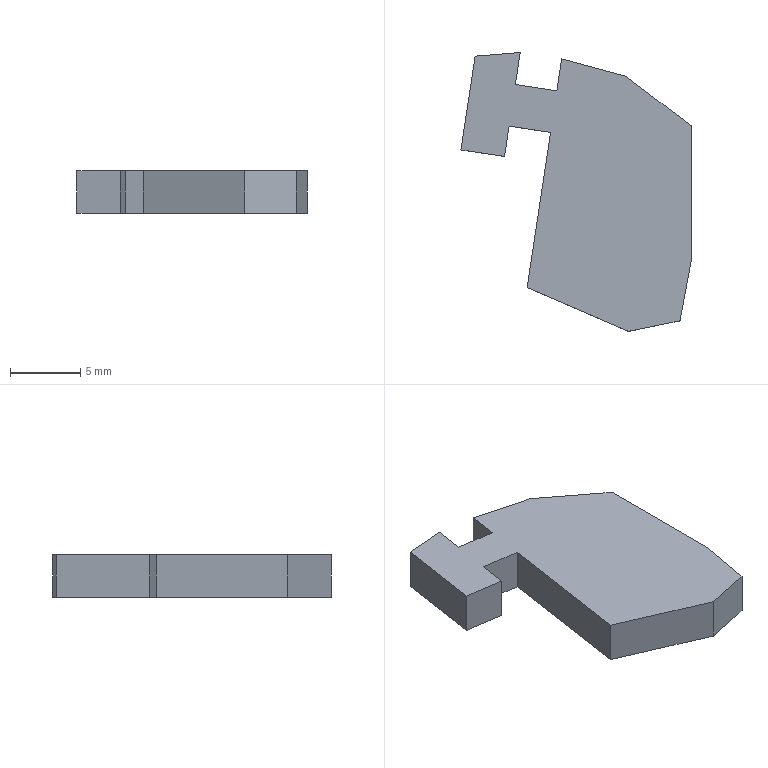Part | SolidWorks | features BaseBody 1 | 1 solid | 17 faces | box 16.417 x 19.898 x 3 mm | volume 620.666 mm3 | plane 17
STEP:
#1=CARTESIAN_POINT('',(6.476,-7.983,-1.5));
#2=VERTEX_POINT('',#1);
#3=CARTESIAN_POINT('',(7.263,-3.747,-1.5));
#4=VERTEX_POINT('',#3);
#5=CARTESIAN_POINT('',(6.476,-7.983,-1.5));
#6=DIRECTION('',(0.1826,0.9832,0.));
#7=VECTOR('',#6,1000.);
#8=LINE('',#5,#7);
#9=EDGE_CURVE('',#2,#4,#8,.T.);
#10=ORIENTED_EDGE('',*,*,#9,.F.);
#11=CARTESIAN_POINT('',(2.819,-8.745,-1.5));
#12=VERTEX_POINT('',#11);
#13=CARTESIAN_POINT('',(2.819,-8.745,-1.5));
#14=DIRECTION('',(0.9789,0.2042,0.));
#15=VECTOR('',#14,1000.);
#16=LINE('',#13,#15);
#17=EDGE_CURVE('',#12,#2,#16,.T.);
#18=ORIENTED_EDGE('',*,*,#17,.F.);
#19=CARTESIAN_POINT('',(-4.433,-5.618,-1.5));
#20=VERTEX_POINT('',#19);
#21=CARTESIAN_POINT('',(-4.433,-5.618,-1.5));
#22=DIRECTION('',(0.9183,-0.3959,0.));
#23=VECTOR('',#22,1000.);
#24=LINE('',#21,#23);
#25=EDGE_CURVE('',#20,#12,#24,.T.);
#26=ORIENTED_EDGE('',*,*,#25,.F.);
#27=CARTESIAN_POINT('',(-2.759,5.455,-1.5));
#28=VERTEX_POINT('',#27);
#29=CARTESIAN_POINT('',(-2.759,5.455,-1.5));
#30=DIRECTION('',(-0.1495,-0.9888,0.));
#31=VECTOR('',#30,1000.);
#32=LINE('',#29,#31);
#33=EDGE_CURVE('',#28,#20,#32,.T.);
#34=ORIENTED_EDGE('',*,*,#33,.F.);
#35=CARTESIAN_POINT('',(-5.721,5.903,-1.5));
#36=VERTEX_POINT('',#35);
#37=CARTESIAN_POINT('',(-5.721,5.903,-1.5));
#38=DIRECTION('',(0.9888,-0.1495,0.));
#39=VECTOR('',#38,1000.);
#40=LINE('',#37,#39);
#41=EDGE_CURVE('',#36,#28,#40,.T.);
#42=ORIENTED_EDGE('',*,*,#41,.F.);
#43=CARTESIAN_POINT('',(-6.049,3.738,-1.5));
#44=VERTEX_POINT('',#43);
#45=CARTESIAN_POINT('',(-6.049,3.738,-1.5));
#46=DIRECTION('',(0.1495,0.9888,0.));
#47=VECTOR('',#46,1000.);
#48=LINE('',#45,#47);
#49=EDGE_CURVE('',#44,#36,#48,.T.);
#50=ORIENTED_EDGE('',*,*,#49,.F.);
#51=CARTESIAN_POINT('',(-9.154,4.206,-1.5));
#52=VERTEX_POINT('',#51);
#53=CARTESIAN_POINT('',(-9.154,4.206,-1.5));
#54=DIRECTION('',(0.9889,-0.1488,0.));
#55=VECTOR('',#54,1000.);
#56=LINE('',#53,#55);
#57=EDGE_CURVE('',#52,#44,#56,.T.);
#58=ORIENTED_EDGE('',*,*,#57,.F.);
#59=CARTESIAN_POINT('',(-8.143,10.895,-1.5));
#60=VERTEX_POINT('',#59);
#61=CARTESIAN_POINT('',(-8.143,10.895,-1.5));
#62=DIRECTION('',(-0.1495,-0.9888,0.));
#63=VECTOR('',#62,1000.);
#64=LINE('',#61,#63);
#65=EDGE_CURVE('',#60,#52,#64,.T.);
#66=ORIENTED_EDGE('',*,*,#65,.F.);
#67=CARTESIAN_POINT('',(-4.928,11.153,-1.5));
#68=VERTEX_POINT('',#67);
#69=CARTESIAN_POINT('',(-4.928,11.153,-1.5));
#70=DIRECTION('',(-0.9968,-0.08003,0.));
#71=VECTOR('',#70,1000.);
#72=LINE('',#69,#71);
#73=EDGE_CURVE('',#68,#60,#72,.T.);
#74=ORIENTED_EDGE('',*,*,#73,.F.);
#75=CARTESIAN_POINT('',(-5.273,8.869,-1.5));
#76=VERTEX_POINT('',#75);
#77=CARTESIAN_POINT('',(-5.273,8.869,-1.5));
#78=DIRECTION('',(0.1495,0.9888,0.));
#79=VECTOR('',#78,1000.);
#80=LINE('',#77,#79);
#81=EDGE_CURVE('',#76,#68,#80,.T.);
#82=ORIENTED_EDGE('',*,*,#81,.F.);
#83=CARTESIAN_POINT('',(-2.31,8.421,-1.5));
#84=VERTEX_POINT('',#83);
#85=CARTESIAN_POINT('',(-2.31,8.421,-1.5));
#86=DIRECTION('',(-0.9888,0.1495,0.));
#87=VECTOR('',#86,1000.);
#88=LINE('',#85,#87);
#89=EDGE_CURVE('',#84,#76,#88,.T.);
#90=ORIENTED_EDGE('',*,*,#89,.F.);
#91=CARTESIAN_POINT('',(-1.965,10.705,-1.5));
#92=VERTEX_POINT('',#91);
#93=CARTESIAN_POINT('',(-2.31,8.421,-1.5));
#94=DIRECTION('',(0.1495,0.9888,0.));
#95=VECTOR('',#94,1000.);
#96=LINE('',#93,#95);
#97=EDGE_CURVE('',#84,#92,#96,.T.);
#98=ORIENTED_EDGE('',*,*,#97,.T.);
#99=CARTESIAN_POINT('',(2.616,9.465,-1.5));
#100=VERTEX_POINT('',#99);
#101=CARTESIAN_POINT('',(2.616,9.465,-1.5));
#102=DIRECTION('',(-0.9652,0.2614,0.));
#103=VECTOR('',#102,1000.);
#104=LINE('',#101,#103);
#105=EDGE_CURVE('',#100,#92,#104,.T.);
#106=ORIENTED_EDGE('',*,*,#105,.F.);
#107=CARTESIAN_POINT('',(7.263,5.919,-1.5));
#108=VERTEX_POINT('',#107);
#109=CARTESIAN_POINT('',(7.263,5.919,-1.5));
#110=DIRECTION('',(-0.795,0.6067,0.));
#111=VECTOR('',#110,1000.);
#112=LINE('',#109,#111);
#113=EDGE_CURVE('',#108,#100,#112,.T.);
#114=ORIENTED_EDGE('',*,*,#113,.F.);
#115=CARTESIAN_POINT('',(7.263,-3.747,-1.5));
#116=DIRECTION('',(0.,1.,0.));
#117=VECTOR('',#116,1000.);
#118=LINE('',#115,#117);
#119=EDGE_CURVE('',#4,#108,#118,.T.);
#120=ORIENTED_EDGE('',*,*,#119,.F.);
#121=EDGE_LOOP('',(#10,#18,#26,#34,#42,#50,#58,#66,#74,#82,#90,#98,#106,#114,#120));
#122=FACE_OUTER_BOUND('',#121,.T.);
#123=CARTESIAN_POINT('',(0.,0.,-1.5));
#124=DIRECTION('',(0.,0.,1.));
#125=DIRECTION('',(1.,0.,0.));
#126=AXIS2_PLACEMENT_3D('',#123,#124,#125);
#127=PLANE('',#126);
#128=ADVANCED_FACE('',(#122),#127,.F.);
#129=CARTESIAN_POINT('',(6.476,-7.983,1.5));
#130=VERTEX_POINT('',#129);
#131=CARTESIAN_POINT('',(7.263,-3.747,1.5));
#132=VERTEX_POINT('',#131);
#133=CARTESIAN_POINT('',(6.476,-7.983,1.5));
#134=DIRECTION('',(0.1826,0.9832,0.));
#135=VECTOR('',#134,1000.);
#136=LINE('',#133,#135);
#137=EDGE_CURVE('',#130,#132,#136,.T.);
#138=ORIENTED_EDGE('',*,*,#137,.T.);
#139=CARTESIAN_POINT('',(7.263,5.919,1.5));
#140=VERTEX_POINT('',#139);
#141=CARTESIAN_POINT('',(7.263,-3.747,1.5));
#142=DIRECTION('',(0.,1.,0.));
#143=VECTOR('',#142,1000.);
#144=LINE('',#141,#143);
#145=EDGE_CURVE('',#132,#140,#144,.T.);
#146=ORIENTED_EDGE('',*,*,#145,.T.);
#147=CARTESIAN_POINT('',(2.616,9.465,1.5));
#148=VERTEX_POINT('',#147);
#149=CARTESIAN_POINT('',(7.263,5.919,1.5));
#150=DIRECTION('',(-0.795,0.6067,0.));
#151=VECTOR('',#150,1000.);
#152=LINE('',#149,#151);
#153=EDGE_CURVE('',#140,#148,#152,.T.);
#154=ORIENTED_EDGE('',*,*,#153,.T.);
#155=CARTESIAN_POINT('',(-1.965,10.705,1.5));
#156=VERTEX_POINT('',#155);
#157=CARTESIAN_POINT('',(2.616,9.465,1.5));
#158=DIRECTION('',(-0.9652,0.2614,0.));
#159=VECTOR('',#158,1000.);
#160=LINE('',#157,#159);
#161=EDGE_CURVE('',#148,#156,#160,.T.);
#162=ORIENTED_EDGE('',*,*,#161,.T.);
#163=CARTESIAN_POINT('',(-2.31,8.421,1.5));
#164=VERTEX_POINT('',#163);
#165=CARTESIAN_POINT('',(-2.31,8.421,1.5));
#166=DIRECTION('',(0.1495,0.9888,0.));
#167=VECTOR('',#166,1000.);
#168=LINE('',#165,#167);
#169=EDGE_CURVE('',#164,#156,#168,.T.);
#170=ORIENTED_EDGE('',*,*,#169,.F.);
#171=CARTESIAN_POINT('',(-5.273,8.869,1.5));
#172=VERTEX_POINT('',#171);
#173=CARTESIAN_POINT('',(-2.31,8.421,1.5));
#174=DIRECTION('',(-0.9888,0.1495,0.));
#175=VECTOR('',#174,1000.);
#176=LINE('',#173,#175);
#177=EDGE_CURVE('',#164,#172,#176,.T.);
#178=ORIENTED_EDGE('',*,*,#177,.T.);
#179=CARTESIAN_POINT('',(-4.928,11.153,1.5));
#180=VERTEX_POINT('',#179);
#181=CARTESIAN_POINT('',(-5.273,8.869,1.5));
#182=DIRECTION('',(0.1495,0.9888,0.));
#183=VECTOR('',#182,1000.);
#184=LINE('',#181,#183);
#185=EDGE_CURVE('',#172,#180,#184,.T.);
#186=ORIENTED_EDGE('',*,*,#185,.T.);
#187=CARTESIAN_POINT('',(-8.143,10.895,1.5));
#188=VERTEX_POINT('',#187);
#189=CARTESIAN_POINT('',(-4.928,11.153,1.5));
#190=DIRECTION('',(-0.9968,-0.08003,0.));
#191=VECTOR('',#190,1000.);
#192=LINE('',#189,#191);
#193=EDGE_CURVE('',#180,#188,#192,.T.);
#194=ORIENTED_EDGE('',*,*,#193,.T.);
#195=CARTESIAN_POINT('',(-9.154,4.206,1.5));
#196=VERTEX_POINT('',#195);
#197=CARTESIAN_POINT('',(-8.143,10.895,1.5));
#198=DIRECTION('',(-0.1495,-0.9888,0.));
#199=VECTOR('',#198,1000.);
#200=LINE('',#197,#199);
#201=EDGE_CURVE('',#188,#196,#200,.T.);
#202=ORIENTED_EDGE('',*,*,#201,.T.);
#203=CARTESIAN_POINT('',(-6.049,3.738,1.5));
#204=VERTEX_POINT('',#203);
#205=CARTESIAN_POINT('',(-9.154,4.206,1.5));
#206=DIRECTION('',(0.9889,-0.1488,0.));
#207=VECTOR('',#206,1000.);
#208=LINE('',#205,#207);
#209=EDGE_CURVE('',#196,#204,#208,.T.);
#210=ORIENTED_EDGE('',*,*,#209,.T.);
#211=CARTESIAN_POINT('',(-5.721,5.903,1.5));
#212=VERTEX_POINT('',#211);
#213=CARTESIAN_POINT('',(-6.049,3.738,1.5));
#214=DIRECTION('',(0.1495,0.9888,0.));
#215=VECTOR('',#214,1000.);
#216=LINE('',#213,#215);
#217=EDGE_CURVE('',#204,#212,#216,.T.);
#218=ORIENTED_EDGE('',*,*,#217,.T.);
#219=CARTESIAN_POINT('',(-2.759,5.455,1.5));
#220=VERTEX_POINT('',#219);
#221=CARTESIAN_POINT('',(-5.721,5.903,1.5));
#222=DIRECTION('',(0.9888,-0.1495,0.));
#223=VECTOR('',#222,1000.);
#224=LINE('',#221,#223);
#225=EDGE_CURVE('',#212,#220,#224,.T.);
#226=ORIENTED_EDGE('',*,*,#225,.T.);
#227=CARTESIAN_POINT('',(-4.433,-5.618,1.5));
#228=VERTEX_POINT('',#227);
#229=CARTESIAN_POINT('',(-2.759,5.455,1.5));
#230=DIRECTION('',(-0.1495,-0.9888,0.));
#231=VECTOR('',#230,1000.);
#232=LINE('',#229,#231);
#233=EDGE_CURVE('',#220,#228,#232,.T.);
#234=ORIENTED_EDGE('',*,*,#233,.T.);
#235=CARTESIAN_POINT('',(2.819,-8.745,1.5));
#236=VERTEX_POINT('',#235);
#237=CARTESIAN_POINT('',(-4.433,-5.618,1.5));
#238=DIRECTION('',(0.9183,-0.3959,0.));
#239=VECTOR('',#238,1000.);
#240=LINE('',#237,#239);
#241=EDGE_CURVE('',#228,#236,#240,.T.);
#242=ORIENTED_EDGE('',*,*,#241,.T.);
#243=CARTESIAN_POINT('',(2.819,-8.745,1.5));
#244=DIRECTION('',(0.9789,0.2042,0.));
#245=VECTOR('',#244,1000.);
#246=LINE('',#243,#245);
#247=EDGE_CURVE('',#236,#130,#246,.T.);
#248=ORIENTED_EDGE('',*,*,#247,.T.);
#249=EDGE_LOOP('',(#138,#146,#154,#162,#170,#178,#186,#194,#202,#210,#218,#226,#234,#242,#248));
#250=FACE_OUTER_BOUND('',#249,.T.);
#251=CARTESIAN_POINT('',(0.,0.,1.5));
#252=DIRECTION('',(0.,0.,1.));
#253=DIRECTION('',(1.,0.,0.));
#254=AXIS2_PLACEMENT_3D('',#251,#252,#253);
#255=PLANE('',#254);
#256=ADVANCED_FACE('',(#250),#255,.T.);
#257=ORIENTED_EDGE('',*,*,#17,.T.);
#258=CARTESIAN_POINT('',(6.476,-7.983,1.5));
#259=DIRECTION('',(0.,0.,-1.));
#260=VECTOR('',#259,1000.);
#261=LINE('',#258,#260);
#262=EDGE_CURVE('',#130,#2,#261,.T.);
#263=ORIENTED_EDGE('',*,*,#262,.F.);
#264=ORIENTED_EDGE('',*,*,#247,.F.);
#265=CARTESIAN_POINT('',(2.819,-8.745,1.5));
#266=DIRECTION('',(0.,0.,-1.));
#267=VECTOR('',#266,1000.);
#268=LINE('',#265,#267);
#269=EDGE_CURVE('',#236,#12,#268,.T.);
#270=ORIENTED_EDGE('',*,*,#269,.T.);
#271=EDGE_LOOP('',(#257,#263,#264,#270));
#272=FACE_OUTER_BOUND('',#271,.T.);
#273=CARTESIAN_POINT('',(2.819,-8.745,1.5));
#274=DIRECTION('',(-0.2042,0.9789,0.));
#275=DIRECTION('',(0.,0.,1.));
#276=AXIS2_PLACEMENT_3D('',#273,#274,#275);
#277=PLANE('',#276);
#278=ADVANCED_FACE('',(#272),#277,.F.);
#279=ORIENTED_EDGE('',*,*,#25,.T.);
#280=ORIENTED_EDGE('',*,*,#269,.F.);
#281=ORIENTED_EDGE('',*,*,#241,.F.);
#282=CARTESIAN_POINT('',(-4.433,-5.618,1.5));
#283=DIRECTION('',(0.,0.,-1.));
#284=VECTOR('',#283,1000.);
#285=LINE('',#282,#284);
#286=EDGE_CURVE('',#228,#20,#285,.T.);
#287=ORIENTED_EDGE('',*,*,#286,.T.);
#288=EDGE_LOOP('',(#279,#280,#281,#287));
#289=FACE_OUTER_BOUND('',#288,.T.);
#290=CARTESIAN_POINT('',(-4.433,-5.618,1.5));
#291=DIRECTION('',(0.3959,0.9183,0.));
#292=DIRECTION('',(0.,0.,-1.));
#293=AXIS2_PLACEMENT_3D('',#290,#291,#292);
#294=PLANE('',#293);
#295=ADVANCED_FACE('',(#289),#294,.F.);
#296=ORIENTED_EDGE('',*,*,#33,.T.);
#297=ORIENTED_EDGE('',*,*,#286,.F.);
#298=ORIENTED_EDGE('',*,*,#233,.F.);
#299=CARTESIAN_POINT('',(-2.759,5.455,1.5));
#300=DIRECTION('',(0.,0.,-1.));
#301=VECTOR('',#300,1000.);
#302=LINE('',#299,#301);
#303=EDGE_CURVE('',#220,#28,#302,.T.);
#304=ORIENTED_EDGE('',*,*,#303,.T.);
#305=EDGE_LOOP('',(#296,#297,#298,#304));
#306=FACE_OUTER_BOUND('',#305,.T.);
#307=CARTESIAN_POINT('',(-2.759,5.455,1.5));
#308=DIRECTION('',(0.9888,-0.1495,0.));
#309=DIRECTION('',(0.,0.,-1.));
#310=AXIS2_PLACEMENT_3D('',#307,#308,#309);
#311=PLANE('',#310);
#312=ADVANCED_FACE('',(#306),#311,.F.);
#313=ORIENTED_EDGE('',*,*,#41,.T.);
#314=ORIENTED_EDGE('',*,*,#303,.F.);
#315=ORIENTED_EDGE('',*,*,#225,.F.);
#316=CARTESIAN_POINT('',(-5.721,5.903,1.5));
#317=DIRECTION('',(0.,0.,-1.));
#318=VECTOR('',#317,1000.);
#319=LINE('',#316,#318);
#320=EDGE_CURVE('',#212,#36,#319,.T.);
#321=ORIENTED_EDGE('',*,*,#320,.T.);
#322=EDGE_LOOP('',(#313,#314,#315,#321));
#323=FACE_OUTER_BOUND('',#322,.T.);
#324=CARTESIAN_POINT('',(-5.721,5.903,1.5));
#325=DIRECTION('',(0.1495,0.9888,0.));
#326=DIRECTION('',(0.,0.,-1.));
#327=AXIS2_PLACEMENT_3D('',#324,#325,#326);
#328=PLANE('',#327);
#329=ADVANCED_FACE('',(#323),#328,.F.);
#330=ORIENTED_EDGE('',*,*,#49,.T.);
#331=ORIENTED_EDGE('',*,*,#320,.F.);
#332=ORIENTED_EDGE('',*,*,#217,.F.);
#333=CARTESIAN_POINT('',(-6.049,3.738,1.5));
#334=DIRECTION('',(0.,0.,-1.));
#335=VECTOR('',#334,1000.);
#336=LINE('',#333,#335);
#337=EDGE_CURVE('',#204,#44,#336,.T.);
#338=ORIENTED_EDGE('',*,*,#337,.T.);
#339=EDGE_LOOP('',(#330,#331,#332,#338));
#340=FACE_OUTER_BOUND('',#339,.T.);
#341=CARTESIAN_POINT('',(-6.049,3.738,1.5));
#342=DIRECTION('',(-0.9888,0.1495,0.));
#343=DIRECTION('',(0.,0.,1.));
#344=AXIS2_PLACEMENT_3D('',#341,#342,#343);
#345=PLANE('',#344);
#346=ADVANCED_FACE('',(#340),#345,.F.);
#347=ORIENTED_EDGE('',*,*,#57,.T.);
#348=ORIENTED_EDGE('',*,*,#337,.F.);
#349=ORIENTED_EDGE('',*,*,#209,.F.);
#350=CARTESIAN_POINT('',(-9.154,4.206,1.5));
#351=DIRECTION('',(0.,0.,-1.));
#352=VECTOR('',#351,1000.);
#353=LINE('',#350,#352);
#354=EDGE_CURVE('',#196,#52,#353,.T.);
#355=ORIENTED_EDGE('',*,*,#354,.T.);
#356=EDGE_LOOP('',(#347,#348,#349,#355));
#357=FACE_OUTER_BOUND('',#356,.T.);
#358=CARTESIAN_POINT('',(-9.154,4.206,1.5));
#359=DIRECTION('',(0.1488,0.9889,0.));
#360=DIRECTION('',(0.,0.,-1.));
#361=AXIS2_PLACEMENT_3D('',#358,#359,#360);
#362=PLANE('',#361);
#363=ADVANCED_FACE('',(#357),#362,.F.);
#364=ORIENTED_EDGE('',*,*,#65,.T.);
#365=ORIENTED_EDGE('',*,*,#354,.F.);
#366=ORIENTED_EDGE('',*,*,#201,.F.);
#367=CARTESIAN_POINT('',(-8.143,10.895,1.5));
#368=DIRECTION('',(0.,0.,-1.));
#369=VECTOR('',#368,1000.);
#370=LINE('',#367,#369);
#371=EDGE_CURVE('',#188,#60,#370,.T.);
#372=ORIENTED_EDGE('',*,*,#371,.T.);
#373=EDGE_LOOP('',(#364,#365,#366,#372));
#374=FACE_OUTER_BOUND('',#373,.T.);
#375=CARTESIAN_POINT('',(-8.143,10.895,1.5));
#376=DIRECTION('',(0.9888,-0.1495,0.));
#377=DIRECTION('',(0.,0.,-1.));
#378=AXIS2_PLACEMENT_3D('',#375,#376,#377);
#379=PLANE('',#378);
#380=ADVANCED_FACE('',(#374),#379,.F.);
#381=ORIENTED_EDGE('',*,*,#73,.T.);
#382=ORIENTED_EDGE('',*,*,#371,.F.);
#383=ORIENTED_EDGE('',*,*,#193,.F.);
#384=CARTESIAN_POINT('',(-4.928,11.153,1.5));
#385=DIRECTION('',(0.,0.,-1.));
#386=VECTOR('',#385,1000.);
#387=LINE('',#384,#386);
#388=EDGE_CURVE('',#180,#68,#387,.T.);
#389=ORIENTED_EDGE('',*,*,#388,.T.);
#390=EDGE_LOOP('',(#381,#382,#383,#389));
#391=FACE_OUTER_BOUND('',#390,.T.);
#392=CARTESIAN_POINT('',(-4.928,11.153,1.5));
#393=DIRECTION('',(0.08003,-0.9968,0.));
#394=DIRECTION('',(0.,0.,-1.));
#395=AXIS2_PLACEMENT_3D('',#392,#393,#394);
#396=PLANE('',#395);
#397=ADVANCED_FACE('',(#391),#396,.F.);
#398=ORIENTED_EDGE('',*,*,#81,.T.);
#399=ORIENTED_EDGE('',*,*,#388,.F.);
#400=ORIENTED_EDGE('',*,*,#185,.F.);
#401=CARTESIAN_POINT('',(-5.273,8.869,1.5));
#402=DIRECTION('',(0.,0.,-1.));
#403=VECTOR('',#402,1000.);
#404=LINE('',#401,#403);
#405=EDGE_CURVE('',#172,#76,#404,.T.);
#406=ORIENTED_EDGE('',*,*,#405,.T.);
#407=EDGE_LOOP('',(#398,#399,#400,#406));
#408=FACE_OUTER_BOUND('',#407,.T.);
#409=CARTESIAN_POINT('',(-5.273,8.869,1.5));
#410=DIRECTION('',(-0.9888,0.1495,0.));
#411=DIRECTION('',(0.,0.,1.));
#412=AXIS2_PLACEMENT_3D('',#409,#410,#411);
#413=PLANE('',#412);
#414=ADVANCED_FACE('',(#408),#413,.F.);
#415=ORIENTED_EDGE('',*,*,#89,.T.);
#416=ORIENTED_EDGE('',*,*,#405,.F.);
#417=ORIENTED_EDGE('',*,*,#177,.F.);
#418=CARTESIAN_POINT('',(-2.31,8.421,1.5));
#419=DIRECTION('',(0.,0.,-1.));
#420=VECTOR('',#419,1000.);
#421=LINE('',#418,#420);
#422=EDGE_CURVE('',#164,#84,#421,.T.);
#423=ORIENTED_EDGE('',*,*,#422,.T.);
#424=EDGE_LOOP('',(#415,#416,#417,#423));
#425=FACE_OUTER_BOUND('',#424,.T.);
#426=CARTESIAN_POINT('',(-2.31,8.421,1.5));
#427=DIRECTION('',(-0.1495,-0.9888,0.));
#428=DIRECTION('',(-0.9888,0.1495,0.));
#429=AXIS2_PLACEMENT_3D('',#426,#427,#428);
#430=PLANE('',#429);
#431=ADVANCED_FACE('',(#425),#430,.F.);
#432=ORIENTED_EDGE('',*,*,#97,.F.);
#433=ORIENTED_EDGE('',*,*,#422,.F.);
#434=ORIENTED_EDGE('',*,*,#169,.T.);
#435=CARTESIAN_POINT('',(-1.965,10.705,1.5));
#436=DIRECTION('',(0.,0.,-1.));
#437=VECTOR('',#436,1000.);
#438=LINE('',#435,#437);
#439=EDGE_CURVE('',#156,#92,#438,.T.);
#440=ORIENTED_EDGE('',*,*,#439,.T.);
#441=EDGE_LOOP('',(#432,#433,#434,#440));
#442=FACE_OUTER_BOUND('',#441,.T.);
#443=CARTESIAN_POINT('',(-2.31,8.421,1.5));
#444=DIRECTION('',(-0.9888,0.1495,0.));
#445=DIRECTION('',(0.,0.,1.));
#446=AXIS2_PLACEMENT_3D('',#443,#444,#445);
#447=PLANE('',#446);
#448=ADVANCED_FACE('',(#442),#447,.T.);
#449=ORIENTED_EDGE('',*,*,#105,.T.);
#450=ORIENTED_EDGE('',*,*,#439,.F.);
#451=ORIENTED_EDGE('',*,*,#161,.F.);
#452=CARTESIAN_POINT('',(2.616,9.465,1.5));
#453=DIRECTION('',(0.,0.,-1.));
#454=VECTOR('',#453,1000.);
#455=LINE('',#452,#454);
#456=EDGE_CURVE('',#148,#100,#455,.T.);
#457=ORIENTED_EDGE('',*,*,#456,.T.);
#458=EDGE_LOOP('',(#449,#450,#451,#457));
#459=FACE_OUTER_BOUND('',#458,.T.);
#460=CARTESIAN_POINT('',(2.616,9.465,1.5));
#461=DIRECTION('',(-0.2614,-0.9652,0.));
#462=DIRECTION('',(-0.9652,0.2614,0.));
#463=AXIS2_PLACEMENT_3D('',#460,#461,#462);
#464=PLANE('',#463);
#465=ADVANCED_FACE('',(#459),#464,.F.);
#466=ORIENTED_EDGE('',*,*,#113,.T.);
#467=ORIENTED_EDGE('',*,*,#456,.F.);
#468=ORIENTED_EDGE('',*,*,#153,.F.);
#469=CARTESIAN_POINT('',(7.263,5.919,1.5));
#470=DIRECTION('',(0.,0.,-1.));
#471=VECTOR('',#470,1000.);
#472=LINE('',#469,#471);
#473=EDGE_CURVE('',#140,#108,#472,.T.);
#474=ORIENTED_EDGE('',*,*,#473,.T.);
#475=EDGE_LOOP('',(#466,#467,#468,#474));
#476=FACE_OUTER_BOUND('',#475,.T.);
#477=CARTESIAN_POINT('',(7.263,5.919,1.5));
#478=DIRECTION('',(-0.6067,-0.795,0.));
#479=DIRECTION('',(-0.795,0.6067,0.));
#480=AXIS2_PLACEMENT_3D('',#477,#478,#479);
#481=PLANE('',#480);
#482=ADVANCED_FACE('',(#476),#481,.F.);
#483=ORIENTED_EDGE('',*,*,#119,.T.);
#484=ORIENTED_EDGE('',*,*,#473,.F.);
#485=ORIENTED_EDGE('',*,*,#145,.F.);
#486=CARTESIAN_POINT('',(7.263,-3.747,1.5));
#487=DIRECTION('',(0.,0.,-1.));
#488=VECTOR('',#487,1000.);
#489=LINE('',#486,#488);
#490=EDGE_CURVE('',#132,#4,#489,.T.);
#491=ORIENTED_EDGE('',*,*,#490,.T.);
#492=EDGE_LOOP('',(#483,#484,#485,#491));
#493=FACE_OUTER_BOUND('',#492,.T.);
#494=CARTESIAN_POINT('',(7.263,-3.747,1.5));
#495=DIRECTION('',(-1.,0.,0.));
#496=DIRECTION('',(0.,0.,1.));
#497=AXIS2_PLACEMENT_3D('',#494,#495,#496);
#498=PLANE('',#497);
#499=ADVANCED_FACE('',(#493),#498,.F.);
#500=ORIENTED_EDGE('',*,*,#9,.T.);
#501=ORIENTED_EDGE('',*,*,#490,.F.);
#502=ORIENTED_EDGE('',*,*,#137,.F.);
#503=ORIENTED_EDGE('',*,*,#262,.T.);
#504=EDGE_LOOP('',(#500,#501,#502,#503));
#505=FACE_OUTER_BOUND('',#504,.T.);
#506=CARTESIAN_POINT('',(6.476,-7.983,1.5));
#507=DIRECTION('',(-0.9832,0.1826,0.));
#508=DIRECTION('',(0.,0.,1.));
#509=AXIS2_PLACEMENT_3D('',#506,#507,#508);
#510=PLANE('',#509);
#511=ADVANCED_FACE('',(#505),#510,.F.);
#512=CLOSED_SHELL('',(#128,#256,#278,#295,#312,#329,#346,#363,#380,#397,#414,#431,#448,#465,#482,#499,#511));
#513=MANIFOLD_SOLID_BREP('',#512);
#514=CARTESIAN_POINT('',(0.,0.,0.));
#515=DIRECTION('',(0.,0.,1.));
#516=DIRECTION('',(1.,0.,0.));
#517=AXIS2_PLACEMENT_3D('',#514,#515,#516);
#518=(LENGTH_UNIT()NAMED_UNIT(*)SI_UNIT(.MILLI.,.METRE.));
#519=UNCERTAINTY_MEASURE_WITH_UNIT(LENGTH_MEASURE(0.00001),#518,'','');
#520=(NAMED_UNIT(*)PLANE_ANGLE_UNIT()SI_UNIT($,.RADIAN.));
#521=(NAMED_UNIT(*)SI_UNIT($,.STERADIAN.)SOLID_ANGLE_UNIT());
#522=(GEOMETRIC_REPRESENTATION_CONTEXT(3)GLOBAL_UNCERTAINTY_ASSIGNED_CONTEXT((#519))GLOBAL_UNIT_ASSIGNED_CONTEXT((#518,#520,#521))REPRESENTATION_CONTEXT('',''));
#523=ADVANCED_BREP_SHAPE_REPRESENTATION('',(#513,#517),#522);